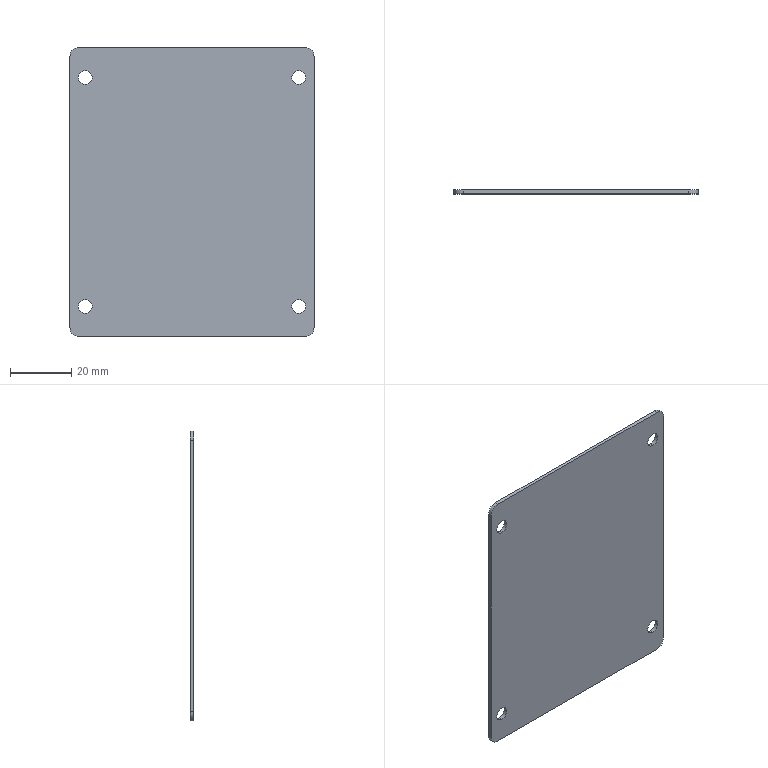Part | STEP file | 1 solid | 18 faces | box 80 x 1.2 x 95 mm | volume 9034 mm3 | cylinder 12 | plane 6 | commonest cylinder face diameters 4.5 x8 6 x4